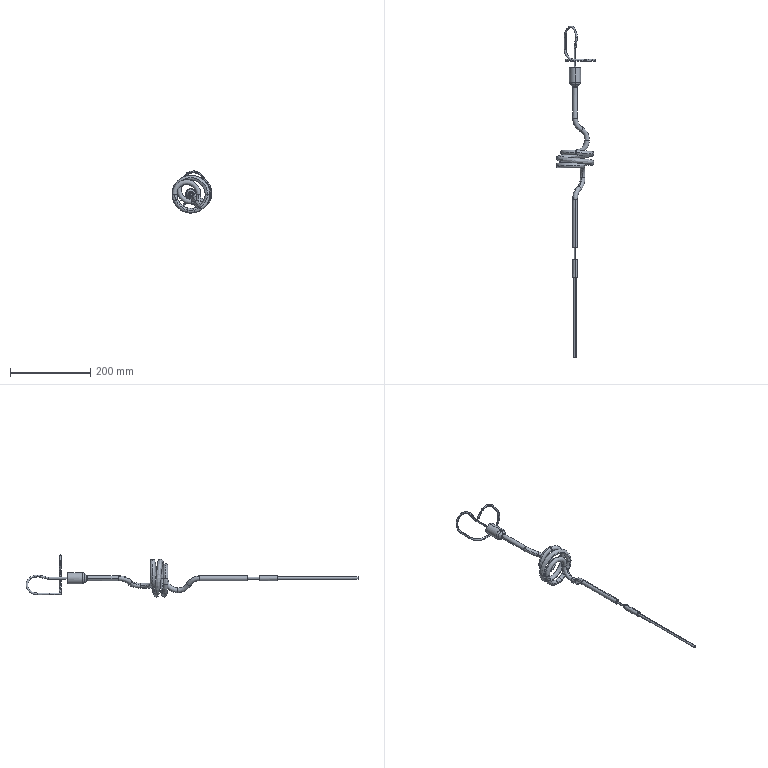Part | NX | features BREP 7 | 5 solids | 252 faces | box 99.502 x 828.984 x 105.44 mm | volume 138294 mm3 | torus 126 | cylinder 64 | spline 25 | plane 21 | cone 16 | commonest cylinder face diameters 4.76 x14 2.322 x13 12 x12 2.337 x9 4.763 x2 6.107 x2